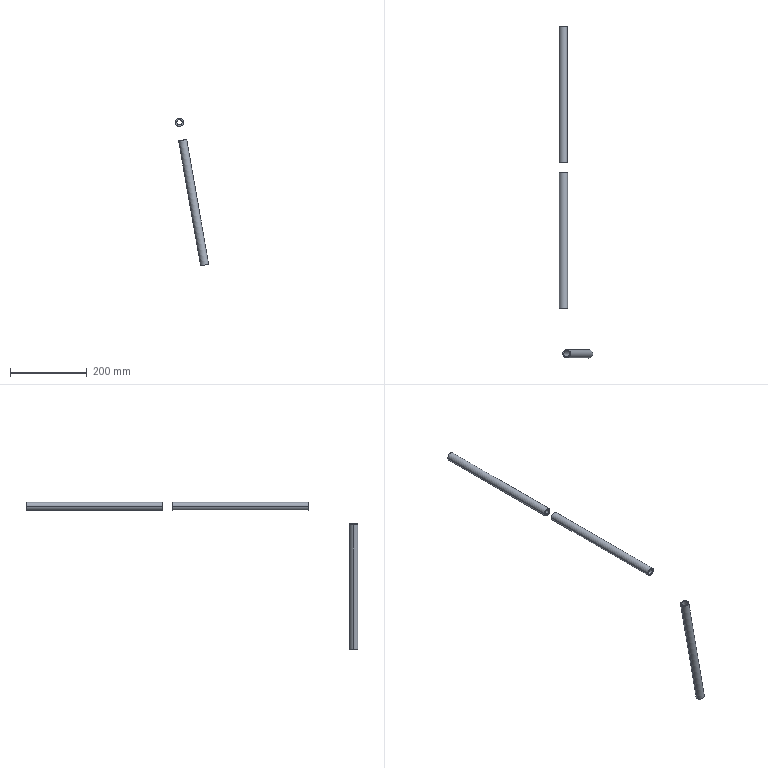Part | SolidWorks | features BaseBody 3 | 3 solids | 18 faces | box 86.694 x 862.008 x 383.174 mm | volume 199579 mm3 | cylinder 10 | plane 6 | spline 2 | commonest cylinder face diameters 21.234 x6 13.868 x2 15.234 x2
STEP:
#1=CARTESIAN_POINT('',(-12.954,392.7,7.));
#2=VERTEX_POINT('',#1);
#3=CARTESIAN_POINT('',(-12.954,392.7,-7.));
#4=VERTEX_POINT('',#3);
#5=CARTESIAN_POINT('',(-12.954,392.7,7.));
#6=CARTESIAN_POINT('',(-13.439,392.7,7.));
#7=CARTESIAN_POINT('',(-13.923,392.7,6.95));
#8=CARTESIAN_POINT('',(-14.398,392.7,6.85));
#9=CARTESIAN_POINT('',(-14.969,392.7,6.729));
#10=CARTESIAN_POINT('',(-15.523,392.7,6.538));
#11=CARTESIAN_POINT('',(-16.047,392.7,6.28));
#12=CARTESIAN_POINT('',(-16.797,392.7,5.91));
#13=CARTESIAN_POINT('',(-17.476,392.7,5.409));
#14=CARTESIAN_POINT('',(-18.049,392.7,4.8));
#15=CARTESIAN_POINT('',(-18.644,392.7,4.168));
#16=CARTESIAN_POINT('',(-19.117,392.7,3.431));
#17=CARTESIAN_POINT('',(-19.442,392.7,2.626));
#18=CARTESIAN_POINT('',(-19.78,392.7,1.792));
#19=CARTESIAN_POINT('',(-19.954,392.7,0.9002));
#20=CARTESIAN_POINT('',(-19.954,392.7,0.));
#21=CARTESIAN_POINT('',(-19.954,392.7,-0.9002));
#22=CARTESIAN_POINT('',(-19.78,392.7,-1.792));
#23=CARTESIAN_POINT('',(-19.442,392.7,-2.626));
#24=CARTESIAN_POINT('',(-19.117,392.7,-3.431));
#25=CARTESIAN_POINT('',(-18.644,392.7,-4.168));
#26=CARTESIAN_POINT('',(-18.049,392.7,-4.8));
#27=CARTESIAN_POINT('',(-17.476,392.7,-5.409));
#28=CARTESIAN_POINT('',(-16.797,392.7,-5.91));
#29=CARTESIAN_POINT('',(-16.047,392.7,-6.28));
#30=CARTESIAN_POINT('',(-15.523,392.7,-6.538));
#31=CARTESIAN_POINT('',(-14.969,392.7,-6.729));
#32=CARTESIAN_POINT('',(-14.398,392.7,-6.85));
#33=CARTESIAN_POINT('',(-13.923,392.7,-6.95));
#34=CARTESIAN_POINT('',(-13.439,392.7,-7.));
#35=CARTESIAN_POINT('',(-12.954,392.7,-7.));
#36=B_SPLINE_CURVE_WITH_KNOTS('',3,(#5,#6,#7,#8,#9,#10,#11,#12,#13,#14,#15,#16,#17,#18,#19,#20,#21,#22,#23,#24,#25,#26,#27,#28,#29,#30,#31,#32,#33,#34,#35),.UNSPECIFIED.,.F.,.F.,(4,3,3,3,3,3,3,3,3,3,4),(0.,0.1457,0.3209,0.572,0.8325,1.103,1.373,1.633,1.885,2.06,2.205),.UNSPECIFIED.);
#37=EDGE_CURVE('',#2,#4,#36,.T.);
#38=ORIENTED_EDGE('',*,*,#37,.F.);
#39=CARTESIAN_POINT('',(-12.954,392.7,-7.));
#40=CARTESIAN_POINT('',(-12.468,392.7,-7.));
#41=CARTESIAN_POINT('',(-11.984,392.7,-6.95));
#42=CARTESIAN_POINT('',(-11.509,392.7,-6.85));
#43=CARTESIAN_POINT('',(-10.938,392.7,-6.729));
#44=CARTESIAN_POINT('',(-10.384,392.7,-6.538));
#45=CARTESIAN_POINT('',(-9.86,392.7,-6.28));
#46=CARTESIAN_POINT('',(-9.11,392.7,-5.91));
#47=CARTESIAN_POINT('',(-8.432,392.7,-5.409));
#48=CARTESIAN_POINT('',(-7.858,392.7,-4.8));
#49=CARTESIAN_POINT('',(-7.263,392.7,-4.168));
#50=CARTESIAN_POINT('',(-6.79,392.7,-3.431));
#51=CARTESIAN_POINT('',(-6.465,392.7,-2.626));
#52=CARTESIAN_POINT('',(-6.127,392.7,-1.792));
#53=CARTESIAN_POINT('',(-5.953,392.7,-0.9002));
#54=CARTESIAN_POINT('',(-5.953,392.7,0.));
#55=CARTESIAN_POINT('',(-5.953,392.7,0.9002));
#56=CARTESIAN_POINT('',(-6.127,392.7,1.792));
#57=CARTESIAN_POINT('',(-6.465,392.7,2.626));
#58=CARTESIAN_POINT('',(-6.79,392.7,3.431));
#59=CARTESIAN_POINT('',(-7.263,392.7,4.168));
#60=CARTESIAN_POINT('',(-7.858,392.7,4.8));
#61=CARTESIAN_POINT('',(-8.432,392.7,5.409));
#62=CARTESIAN_POINT('',(-9.11,392.7,5.91));
#63=CARTESIAN_POINT('',(-9.86,392.7,6.28));
#64=CARTESIAN_POINT('',(-10.384,392.7,6.538));
#65=CARTESIAN_POINT('',(-10.938,392.7,6.729));
#66=CARTESIAN_POINT('',(-11.509,392.7,6.85));
#67=CARTESIAN_POINT('',(-11.984,392.7,6.95));
#68=CARTESIAN_POINT('',(-12.468,392.7,7.));
#69=CARTESIAN_POINT('',(-12.954,392.7,7.));
#70=B_SPLINE_CURVE_WITH_KNOTS('',3,(#39,#40,#41,#42,#43,#44,#45,#46,#47,#48,#49,#50,#51,#52,#53,#54,#55,#56,#57,#58,#59,#60,#61,#62,#63,#64,#65,#66,#67,#68,#69),.UNSPECIFIED.,.F.,.F.,(4,3,3,3,3,3,3,3,3,3,4),(0.,0.1457,0.3209,0.572,0.8325,1.103,1.373,1.633,1.885,2.06,2.205),.UNSPECIFIED.);
#71=EDGE_CURVE('',#4,#2,#70,.T.);
#72=ORIENTED_EDGE('',*,*,#71,.F.);
#73=EDGE_LOOP('',(#38,#72));
#74=FACE_BOUND('',#73,.T.);
#75=CARTESIAN_POINT('',(-2.337,392.7,0.));
#76=VERTEX_POINT('',#75);
#77=CARTESIAN_POINT('',(-23.571,392.7,0.));
#78=VERTEX_POINT('',#77);
#79=CARTESIAN_POINT('',(-12.954,392.7,0.));
#80=DIRECTION('',(0.,1.,0.));
#81=DIRECTION('',(1.,0.,0.));
#82=AXIS2_PLACEMENT_3D('',#79,#80,#81);
#83=CIRCLE('',#82,10.617);
#84=EDGE_CURVE('',#76,#78,#83,.T.);
#85=ORIENTED_EDGE('',*,*,#84,.F.);
#86=CARTESIAN_POINT('',(-12.954,392.7,0.));
#87=DIRECTION('',(0.,1.,0.));
#88=DIRECTION('',(-1.,0.,0.));
#89=AXIS2_PLACEMENT_3D('',#86,#87,#88);
#90=CIRCLE('',#89,10.617);
#91=EDGE_CURVE('',#78,#76,#90,.T.);
#92=ORIENTED_EDGE('',*,*,#91,.F.);
#93=EDGE_LOOP('',(#85,#92));
#94=FACE_OUTER_BOUND('',#93,.T.);
#95=CARTESIAN_POINT('',(-12.954,392.7,0.));
#96=DIRECTION('',(0.,-1.,0.));
#97=DIRECTION('',(0.,0.,-1.));
#98=AXIS2_PLACEMENT_3D('',#95,#96,#97);
#99=PLANE('',#98);
#100=ADVANCED_FACE('',(#74,#94),#99,.T.);
#101=CARTESIAN_POINT('',(-12.954,747.046,7.));
#102=VERTEX_POINT('',#101);
#103=CARTESIAN_POINT('',(-12.954,747.046,-7.));
#104=VERTEX_POINT('',#103);
#105=CARTESIAN_POINT('',(-12.954,747.046,7.));
#106=CARTESIAN_POINT('',(-12.468,747.046,7.));
#107=CARTESIAN_POINT('',(-11.984,747.046,6.95));
#108=CARTESIAN_POINT('',(-10.938,747.046,6.729));
#109=CARTESIAN_POINT('',(-10.384,747.046,6.538));
#110=CARTESIAN_POINT('',(-9.11,747.046,5.91));
#111=CARTESIAN_POINT('',(-8.432,747.046,5.409));
#112=CARTESIAN_POINT('',(-7.263,747.046,4.168));
#113=CARTESIAN_POINT('',(-6.79,747.046,3.431));
#114=CARTESIAN_POINT('',(-6.127,747.046,1.792));
#115=CARTESIAN_POINT('',(-5.953,747.046,0.9002));
#116=CARTESIAN_POINT('',(-5.953,747.046,-0.9002));
#117=CARTESIAN_POINT('',(-6.127,747.046,-1.792));
#118=CARTESIAN_POINT('',(-6.79,747.046,-3.431));
#119=CARTESIAN_POINT('',(-7.263,747.046,-4.168));
#120=CARTESIAN_POINT('',(-8.432,747.046,-5.409));
#121=CARTESIAN_POINT('',(-9.11,747.046,-5.91));
#122=CARTESIAN_POINT('',(-10.384,747.046,-6.538));
#123=CARTESIAN_POINT('',(-10.938,747.046,-6.729));
#124=CARTESIAN_POINT('',(-11.984,747.046,-6.95));
#125=CARTESIAN_POINT('',(-12.468,747.046,-7.));
#126=CARTESIAN_POINT('',(-12.954,747.046,-7.));
#127=B_SPLINE_CURVE_WITH_KNOTS('',3,(#105,#106,#107,#108,#109,#110,#111,#112,#113,#114,#115,#116,#117,#118,#119,#120,#121,#122,#123,#124,#125,#126),.UNSPECIFIED.,.F.,.F.,(4,2,2,2,2,2,2,2,2,2,4),(0.,0.1456,0.3207,0.5718,0.8321,1.102,1.372,1.633,1.884,2.059,2.204),.UNSPECIFIED.);
#128=EDGE_CURVE('',#102,#104,#127,.T.);
#129=ORIENTED_EDGE('',*,*,#128,.F.);
#130=CARTESIAN_POINT('',(-12.954,747.046,-7.));
#131=CARTESIAN_POINT('',(-13.439,747.046,-7.));
#132=CARTESIAN_POINT('',(-13.923,747.046,-6.95));
#133=CARTESIAN_POINT('',(-14.398,747.046,-6.85));
#134=CARTESIAN_POINT('',(-14.969,747.046,-6.729));
#135=CARTESIAN_POINT('',(-15.523,747.046,-6.538));
#136=CARTESIAN_POINT('',(-16.047,747.046,-6.28));
#137=CARTESIAN_POINT('',(-16.797,747.046,-5.91));
#138=CARTESIAN_POINT('',(-17.476,747.046,-5.409));
#139=CARTESIAN_POINT('',(-18.049,747.046,-4.8));
#140=CARTESIAN_POINT('',(-18.644,747.046,-4.168));
#141=CARTESIAN_POINT('',(-19.117,747.046,-3.431));
#142=CARTESIAN_POINT('',(-19.442,747.046,-2.626));
#143=CARTESIAN_POINT('',(-19.78,747.046,-1.792));
#144=CARTESIAN_POINT('',(-19.954,747.046,-0.9002));
#145=CARTESIAN_POINT('',(-19.954,747.046,0.));
#146=CARTESIAN_POINT('',(-19.954,747.046,0.9002));
#147=CARTESIAN_POINT('',(-19.78,747.046,1.792));
#148=CARTESIAN_POINT('',(-19.442,747.046,2.626));
#149=CARTESIAN_POINT('',(-19.117,747.046,3.431));
#150=CARTESIAN_POINT('',(-18.644,747.046,4.168));
#151=CARTESIAN_POINT('',(-18.049,747.046,4.8));
#152=CARTESIAN_POINT('',(-17.476,747.046,5.409));
#153=CARTESIAN_POINT('',(-16.797,747.046,5.91));
#154=CARTESIAN_POINT('',(-16.047,747.046,6.28));
#155=CARTESIAN_POINT('',(-15.523,747.046,6.538));
#156=CARTESIAN_POINT('',(-14.969,747.046,6.729));
#157=CARTESIAN_POINT('',(-14.398,747.046,6.85));
#158=CARTESIAN_POINT('',(-13.923,747.046,6.95));
#159=CARTESIAN_POINT('',(-13.439,747.046,7.));
#160=CARTESIAN_POINT('',(-12.954,747.046,7.));
#161=B_SPLINE_CURVE_WITH_KNOTS('',3,(#130,#131,#132,#133,#134,#135,#136,#137,#138,#139,#140,#141,#142,#143,#144,#145,#146,#147,#148,#149,#150,#151,#152,#153,#154,#155,#156,#157,#158,#159,#160),.UNSPECIFIED.,.F.,.F.,(4,3,3,3,3,3,3,3,3,3,4),(0.,0.1456,0.3207,0.5718,0.8321,1.102,1.372,1.633,1.884,2.059,2.204),.UNSPECIFIED.);
#162=EDGE_CURVE('',#104,#102,#161,.T.);
#163=ORIENTED_EDGE('',*,*,#162,.F.);
#164=EDGE_LOOP('',(#129,#163));
#165=FACE_BOUND('',#164,.T.);
#166=CARTESIAN_POINT('',(-2.337,747.046,0.));
#167=VERTEX_POINT('',#166);
#168=CARTESIAN_POINT('',(-23.571,747.046,0.));
#169=VERTEX_POINT('',#168);
#170=CARTESIAN_POINT('',(-12.954,747.046,0.));
#171=DIRECTION('',(0.,-1.,0.));
#172=DIRECTION('',(1.,0.,0.));
#173=AXIS2_PLACEMENT_3D('',#170,#171,#172);
#174=CIRCLE('',#173,10.617);
#175=EDGE_CURVE('',#167,#169,#174,.T.);
#176=ORIENTED_EDGE('',*,*,#175,.F.);
#177=CARTESIAN_POINT('',(-12.954,747.046,0.));
#178=DIRECTION('',(0.,-1.,0.));
#179=DIRECTION('',(-1.,0.,0.));
#180=AXIS2_PLACEMENT_3D('',#177,#178,#179);
#181=CIRCLE('',#180,10.617);
#182=EDGE_CURVE('',#169,#167,#181,.T.);
#183=ORIENTED_EDGE('',*,*,#182,.F.);
#184=EDGE_LOOP('',(#176,#183));
#185=FACE_OUTER_BOUND('',#184,.T.);
#186=CARTESIAN_POINT('',(-12.954,747.046,0.));
#187=DIRECTION('',(0.,1.,0.));
#188=DIRECTION('',(1.,0.,0.));
#189=AXIS2_PLACEMENT_3D('',#186,#187,#188);
#190=PLANE('',#189);
#191=ADVANCED_FACE('',(#165,#185),#190,.T.);
#192=ORIENTED_EDGE('',*,*,#71,.T.);
#193=CARTESIAN_POINT('',(-12.954,747.046,7.));
#194=DIRECTION('',(0.,-1.,0.));
#195=VECTOR('',#194,1000.);
#196=LINE('',#193,#195);
#197=EDGE_CURVE('',#102,#2,#196,.T.);
#198=ORIENTED_EDGE('',*,*,#197,.F.);
#199=ORIENTED_EDGE('',*,*,#128,.T.);
#200=CARTESIAN_POINT('',(-12.954,392.7,-7.));
#201=DIRECTION('',(0.,1.,0.));
#202=VECTOR('',#201,1000.);
#203=LINE('',#200,#202);
#204=EDGE_CURVE('',#4,#104,#203,.T.);
#205=ORIENTED_EDGE('',*,*,#204,.F.);
#206=EDGE_LOOP('',(#192,#198,#199,#205));
#207=FACE_OUTER_BOUND('',#206,.T.);
#208=CARTESIAN_POINT('',(-12.954,747.046,7.));
#209=CARTESIAN_POINT('',(-12.954,357.265,7.));
#210=CARTESIAN_POINT('',(-12.468,747.046,7.));
#211=CARTESIAN_POINT('',(-12.468,357.265,7.));
#212=CARTESIAN_POINT('',(-11.984,747.046,6.95));
#213=CARTESIAN_POINT('',(-11.984,357.265,6.95));
#214=CARTESIAN_POINT('',(-10.938,747.046,6.729));
#215=CARTESIAN_POINT('',(-10.938,357.265,6.729));
#216=CARTESIAN_POINT('',(-10.384,747.046,6.538));
#217=CARTESIAN_POINT('',(-10.384,357.265,6.538));
#218=CARTESIAN_POINT('',(-9.11,747.046,5.91));
#219=CARTESIAN_POINT('',(-9.11,357.265,5.91));
#220=CARTESIAN_POINT('',(-8.432,747.046,5.409));
#221=CARTESIAN_POINT('',(-8.432,357.265,5.409));
#222=CARTESIAN_POINT('',(-7.263,747.046,4.168));
#223=CARTESIAN_POINT('',(-7.263,357.265,4.168));
#224=CARTESIAN_POINT('',(-6.79,747.046,3.431));
#225=CARTESIAN_POINT('',(-6.79,357.265,3.431));
#226=CARTESIAN_POINT('',(-6.127,747.046,1.792));
#227=CARTESIAN_POINT('',(-6.127,357.265,1.792));
#228=CARTESIAN_POINT('',(-5.953,747.046,0.9002));
#229=CARTESIAN_POINT('',(-5.953,357.265,0.9002));
#230=CARTESIAN_POINT('',(-5.953,747.046,-0.9002));
#231=CARTESIAN_POINT('',(-5.953,357.265,-0.9002));
#232=CARTESIAN_POINT('',(-6.127,747.046,-1.792));
#233=CARTESIAN_POINT('',(-6.127,357.265,-1.792));
#234=CARTESIAN_POINT('',(-6.79,747.046,-3.431));
#235=CARTESIAN_POINT('',(-6.79,357.265,-3.431));
#236=CARTESIAN_POINT('',(-7.263,747.046,-4.168));
#237=CARTESIAN_POINT('',(-7.263,357.265,-4.168));
#238=CARTESIAN_POINT('',(-8.432,747.046,-5.409));
#239=CARTESIAN_POINT('',(-8.432,357.265,-5.409));
#240=CARTESIAN_POINT('',(-9.11,747.046,-5.91));
#241=CARTESIAN_POINT('',(-9.11,357.265,-5.91));
#242=CARTESIAN_POINT('',(-10.384,747.046,-6.538));
#243=CARTESIAN_POINT('',(-10.384,357.265,-6.538));
#244=CARTESIAN_POINT('',(-10.938,747.046,-6.729));
#245=CARTESIAN_POINT('',(-10.938,357.265,-6.729));
#246=CARTESIAN_POINT('',(-11.984,747.046,-6.95));
#247=CARTESIAN_POINT('',(-11.984,357.265,-6.95));
#248=CARTESIAN_POINT('',(-12.468,747.046,-7.));
#249=CARTESIAN_POINT('',(-12.468,357.265,-7.));
#250=CARTESIAN_POINT('',(-12.954,747.046,-7.));
#251=CARTESIAN_POINT('',(-12.954,357.265,-7.));
#252=B_SPLINE_SURFACE_WITH_KNOTS('',3,1,((#208,#209),(#210,#211),(#212,#213),(#214,#215),(#216,#217),(#218,#219),(#220,#221),(#222,#223),(#224,#225),(#226,#227),(#228,#229),(#230,#231),(#232,#233),(#234,#235),(#236,#237),(#238,#239),(#240,#241),(#242,#243),(#244,#245),(#246,#247),(#248,#249),(#250,#251)),.UNSPECIFIED.,.F.,.F.,.F.,(4,2,2,2,2,2,2,2,2,2,4),(2,2),(0.000001,0.1456,0.3207,0.5718,0.8321,1.102,1.372,1.633,1.884,2.059,2.204),(0.,38.978),.UNSPECIFIED.);
#253=ADVANCED_FACE('',(#207),#252,.T.);
#254=ORIENTED_EDGE('',*,*,#91,.T.);
#255=CARTESIAN_POINT('',(-2.337,747.046,0.));
#256=DIRECTION('',(0.,-1.,0.));
#257=VECTOR('',#256,1000.);
#258=LINE('',#255,#257);
#259=EDGE_CURVE('',#167,#76,#258,.T.);
#260=ORIENTED_EDGE('',*,*,#259,.F.);
#261=ORIENTED_EDGE('',*,*,#175,.T.);
#262=CARTESIAN_POINT('',(-23.571,392.7,0.));
#263=DIRECTION('',(0.,1.,0.));
#264=VECTOR('',#263,1000.);
#265=LINE('',#262,#264);
#266=EDGE_CURVE('',#78,#169,#265,.T.);
#267=ORIENTED_EDGE('',*,*,#266,.F.);
#268=EDGE_LOOP('',(#254,#260,#261,#267));
#269=FACE_OUTER_BOUND('',#268,.T.);
#270=CARTESIAN_POINT('',(-12.954,747.046,0.));
#271=DIRECTION('',(0.,-1.,0.));
#272=DIRECTION('',(1.,0.,0.));
#273=AXIS2_PLACEMENT_3D('',#270,#271,#272);
#274=CYLINDRICAL_SURFACE('',#273,10.617);
#275=ADVANCED_FACE('',(#269),#274,.T.);
#276=ORIENTED_EDGE('',*,*,#266,.T.);
#277=ORIENTED_EDGE('',*,*,#182,.T.);
#278=ORIENTED_EDGE('',*,*,#259,.T.);
#279=ORIENTED_EDGE('',*,*,#84,.T.);
#280=EDGE_LOOP('',(#276,#277,#278,#279));
#281=FACE_OUTER_BOUND('',#280,.T.);
#282=CARTESIAN_POINT('',(-12.954,747.046,0.));
#283=DIRECTION('',(0.,-1.,0.));
#284=DIRECTION('',(1.,0.,0.));
#285=AXIS2_PLACEMENT_3D('',#282,#283,#284);
#286=CYLINDRICAL_SURFACE('',#285,10.617);
#287=ADVANCED_FACE('',(#281),#286,.T.);
#288=ORIENTED_EDGE('',*,*,#37,.T.);
#289=ORIENTED_EDGE('',*,*,#204,.T.);
#290=ORIENTED_EDGE('',*,*,#162,.T.);
#291=ORIENTED_EDGE('',*,*,#197,.T.);
#292=EDGE_LOOP('',(#288,#289,#290,#291));
#293=FACE_OUTER_BOUND('',#292,.T.);
#294=CARTESIAN_POINT('',(-12.954,747.046,-7.));
#295=CARTESIAN_POINT('',(-12.954,357.265,-7.));
#296=CARTESIAN_POINT('',(-13.439,747.046,-7.));
#297=CARTESIAN_POINT('',(-13.439,357.265,-7.));
#298=CARTESIAN_POINT('',(-13.923,747.046,-6.95));
#299=CARTESIAN_POINT('',(-13.923,357.265,-6.95));
#300=CARTESIAN_POINT('',(-14.969,747.046,-6.729));
#301=CARTESIAN_POINT('',(-14.969,357.265,-6.729));
#302=CARTESIAN_POINT('',(-15.523,747.046,-6.538));
#303=CARTESIAN_POINT('',(-15.523,357.265,-6.538));
#304=CARTESIAN_POINT('',(-16.797,747.046,-5.91));
#305=CARTESIAN_POINT('',(-16.797,357.265,-5.91));
#306=CARTESIAN_POINT('',(-17.476,747.046,-5.409));
#307=CARTESIAN_POINT('',(-17.476,357.265,-5.409));
#308=CARTESIAN_POINT('',(-18.644,747.046,-4.168));
#309=CARTESIAN_POINT('',(-18.644,357.265,-4.168));
#310=CARTESIAN_POINT('',(-19.117,747.046,-3.431));
#311=CARTESIAN_POINT('',(-19.117,357.265,-3.431));
#312=CARTESIAN_POINT('',(-19.78,747.046,-1.792));
#313=CARTESIAN_POINT('',(-19.78,357.265,-1.792));
#314=CARTESIAN_POINT('',(-19.954,747.046,-0.9002));
#315=CARTESIAN_POINT('',(-19.954,357.265,-0.9002));
#316=CARTESIAN_POINT('',(-19.954,747.046,0.9002));
#317=CARTESIAN_POINT('',(-19.954,357.265,0.9002));
#318=CARTESIAN_POINT('',(-19.78,747.046,1.792));
#319=CARTESIAN_POINT('',(-19.78,357.265,1.792));
#320=CARTESIAN_POINT('',(-19.117,747.046,3.431));
#321=CARTESIAN_POINT('',(-19.117,357.265,3.431));
#322=CARTESIAN_POINT('',(-18.644,747.046,4.168));
#323=CARTESIAN_POINT('',(-18.644,357.265,4.168));
#324=CARTESIAN_POINT('',(-17.476,747.046,5.409));
#325=CARTESIAN_POINT('',(-17.476,357.265,5.409));
#326=CARTESIAN_POINT('',(-16.797,747.046,5.91));
#327=CARTESIAN_POINT('',(-16.797,357.265,5.91));
#328=CARTESIAN_POINT('',(-15.523,747.046,6.538));
#329=CARTESIAN_POINT('',(-15.523,357.265,6.538));
#330=CARTESIAN_POINT('',(-14.969,747.046,6.729));
#331=CARTESIAN_POINT('',(-14.969,357.265,6.729));
#332=CARTESIAN_POINT('',(-13.923,747.046,6.95));
#333=CARTESIAN_POINT('',(-13.923,357.265,6.95));
#334=CARTESIAN_POINT('',(-13.439,747.046,7.));
#335=CARTESIAN_POINT('',(-13.439,357.265,7.));
#336=CARTESIAN_POINT('',(-12.954,747.046,7.));
#337=CARTESIAN_POINT('',(-12.954,357.265,7.));
#338=B_SPLINE_SURFACE_WITH_KNOTS('',3,1,((#294,#295),(#296,#297),(#298,#299),(#300,#301),(#302,#303),(#304,#305),(#306,#307),(#308,#309),(#310,#311),(#312,#313),(#314,#315),(#316,#317),(#318,#319),(#320,#321),(#322,#323),(#324,#325),(#326,#327),(#328,#329),(#330,#331),(#332,#333),(#334,#335),(#336,#337)),.UNSPECIFIED.,.F.,.F.,.F.,(4,2,2,2,2,2,2,2,2,2,4),(2,2),(0.000001,0.1456,0.3207,0.5718,0.8321,1.102,1.372,1.633,1.884,2.059,2.204),(0.,38.978),.UNSPECIFIED.);
#339=ADVANCED_FACE('',(#293),#338,.T.);
#340=CLOSED_SHELL('',(#100,#191,#253,#275,#287,#339));
#341=MANIFOLD_SOLID_BREP('',#340);
#342=CARTESIAN_POINT('',(-5.766,12.7,0.));
#343=VERTEX_POINT('',#342);
#344=CARTESIAN_POINT('',(-19.634,12.7,0.));
#345=VERTEX_POINT('',#344);
#346=CARTESIAN_POINT('',(-12.7,12.7,0.));
#347=DIRECTION('',(0.,-1.,0.));
#348=DIRECTION('',(1.,0.,0.));
#349=AXIS2_PLACEMENT_3D('',#346,#347,#348);
#350=CIRCLE('',#349,6.934);
#351=EDGE_CURVE('',#343,#345,#350,.T.);
#352=ORIENTED_EDGE('',*,*,#351,.F.);
#353=CARTESIAN_POINT('',(-12.7,12.7,0.));
#354=DIRECTION('',(0.,-1.,0.));
#355=DIRECTION('',(-1.,0.,0.));
#356=AXIS2_PLACEMENT_3D('',#353,#354,#355);
#357=CIRCLE('',#356,6.934);
#358=EDGE_CURVE('',#345,#343,#357,.T.);
#359=ORIENTED_EDGE('',*,*,#358,.F.);
#360=EDGE_LOOP('',(#352,#359));
#361=FACE_BOUND('',#360,.T.);
#362=CARTESIAN_POINT('',(-2.083,12.7,0.));
#363=VERTEX_POINT('',#362);
#364=CARTESIAN_POINT('',(-23.317,12.7,0.));
#365=VERTEX_POINT('',#364);
#366=CARTESIAN_POINT('',(-12.7,12.7,0.));
#367=DIRECTION('',(0.,1.,0.));
#368=DIRECTION('',(1.,0.,0.));
#369=AXIS2_PLACEMENT_3D('',#366,#367,#368);
#370=CIRCLE('',#369,10.617);
#371=EDGE_CURVE('',#363,#365,#370,.T.);
#372=ORIENTED_EDGE('',*,*,#371,.F.);
#373=CARTESIAN_POINT('',(-12.7,12.7,0.));
#374=DIRECTION('',(0.,1.,0.));
#375=DIRECTION('',(-1.,0.,0.));
#376=AXIS2_PLACEMENT_3D('',#373,#374,#375);
#377=CIRCLE('',#376,10.617);
#378=EDGE_CURVE('',#365,#363,#377,.T.);
#379=ORIENTED_EDGE('',*,*,#378,.F.);
#380=EDGE_LOOP('',(#372,#379));
#381=FACE_OUTER_BOUND('',#380,.T.);
#382=CARTESIAN_POINT('',(-12.7,12.7,0.));
#383=DIRECTION('',(0.,-1.,0.));
#384=DIRECTION('',(0.,0.,-1.));
#385=AXIS2_PLACEMENT_3D('',#382,#383,#384);
#386=PLANE('',#385);
#387=ADVANCED_FACE('',(#361,#381),#386,.T.);
#388=CARTESIAN_POINT('',(-5.766,367.3,0.));
#389=VERTEX_POINT('',#388);
#390=CARTESIAN_POINT('',(-19.634,367.3,0.));
#391=VERTEX_POINT('',#390);
#392=CARTESIAN_POINT('',(-12.7,367.3,0.));
#393=DIRECTION('',(0.,1.,0.));
#394=DIRECTION('',(1.,0.,0.));
#395=AXIS2_PLACEMENT_3D('',#392,#393,#394);
#396=CIRCLE('',#395,6.934);
#397=EDGE_CURVE('',#389,#391,#396,.T.);
#398=ORIENTED_EDGE('',*,*,#397,.F.);
#399=CARTESIAN_POINT('',(-12.7,367.3,0.));
#400=DIRECTION('',(0.,1.,0.));
#401=DIRECTION('',(-1.,0.,0.));
#402=AXIS2_PLACEMENT_3D('',#399,#400,#401);
#403=CIRCLE('',#402,6.934);
#404=EDGE_CURVE('',#391,#389,#403,.T.);
#405=ORIENTED_EDGE('',*,*,#404,.F.);
#406=EDGE_LOOP('',(#398,#405));
#407=FACE_BOUND('',#406,.T.);
#408=CARTESIAN_POINT('',(-2.083,367.3,0.));
#409=VERTEX_POINT('',#408);
#410=CARTESIAN_POINT('',(-23.317,367.3,0.));
#411=VERTEX_POINT('',#410);
#412=CARTESIAN_POINT('',(-12.7,367.3,0.));
#413=DIRECTION('',(0.,-1.,0.));
#414=DIRECTION('',(1.,0.,0.));
#415=AXIS2_PLACEMENT_3D('',#412,#413,#414);
#416=CIRCLE('',#415,10.617);
#417=EDGE_CURVE('',#409,#411,#416,.T.);
#418=ORIENTED_EDGE('',*,*,#417,.F.);
#419=CARTESIAN_POINT('',(-12.7,367.3,0.));
#420=DIRECTION('',(0.,-1.,0.));
#421=DIRECTION('',(-1.,0.,0.));
#422=AXIS2_PLACEMENT_3D('',#419,#420,#421);
#423=CIRCLE('',#422,10.617);
#424=EDGE_CURVE('',#411,#409,#423,.T.);
#425=ORIENTED_EDGE('',*,*,#424,.F.);
#426=EDGE_LOOP('',(#418,#425));
#427=FACE_OUTER_BOUND('',#426,.T.);
#428=CARTESIAN_POINT('',(-12.7,367.3,0.));
#429=DIRECTION('',(0.,1.,0.));
#430=DIRECTION('',(1.,0.,0.));
#431=AXIS2_PLACEMENT_3D('',#428,#429,#430);
#432=PLANE('',#431);
#433=ADVANCED_FACE('',(#407,#427),#432,.T.);
#434=ORIENTED_EDGE('',*,*,#378,.T.);
#435=CARTESIAN_POINT('',(-2.083,367.3,0.));
#436=DIRECTION('',(0.,-1.,0.));
#437=VECTOR('',#436,1000.);
#438=LINE('',#435,#437);
#439=EDGE_CURVE('',#409,#363,#438,.T.);
#440=ORIENTED_EDGE('',*,*,#439,.F.);
#441=ORIENTED_EDGE('',*,*,#417,.T.);
#442=CARTESIAN_POINT('',(-23.317,12.7,0.));
#443=DIRECTION('',(0.,1.,0.));
#444=VECTOR('',#443,1000.);
#445=LINE('',#442,#444);
#446=EDGE_CURVE('',#365,#411,#445,.T.);
#447=ORIENTED_EDGE('',*,*,#446,.F.);
#448=EDGE_LOOP('',(#434,#440,#441,#447));
#449=FACE_OUTER_BOUND('',#448,.T.);
#450=CARTESIAN_POINT('',(-12.7,367.3,0.));
#451=DIRECTION('',(0.,-1.,0.));
#452=DIRECTION('',(1.,0.,0.));
#453=AXIS2_PLACEMENT_3D('',#450,#451,#452);
#454=CYLINDRICAL_SURFACE('',#453,10.617);
#455=ADVANCED_FACE('',(#449),#454,.T.);
#456=ORIENTED_EDGE('',*,*,#446,.T.);
#457=ORIENTED_EDGE('',*,*,#424,.T.);
#458=ORIENTED_EDGE('',*,*,#439,.T.);
#459=ORIENTED_EDGE('',*,*,#371,.T.);
#460=EDGE_LOOP('',(#456,#457,#458,#459));
#461=FACE_OUTER_BOUND('',#460,.T.);
#462=CARTESIAN_POINT('',(-12.7,367.3,0.));
#463=DIRECTION('',(0.,-1.,0.));
#464=DIRECTION('',(1.,0.,0.));
#465=AXIS2_PLACEMENT_3D('',#462,#463,#464);
#466=CYLINDRICAL_SURFACE('',#465,10.617);
#467=ADVANCED_FACE('',(#461),#466,.T.);
#468=ORIENTED_EDGE('',*,*,#358,.T.);
#469=CARTESIAN_POINT('',(-5.766,367.3,0.));
#470=DIRECTION('',(0.,-1.,0.));
#471=VECTOR('',#470,1000.);
#472=LINE('',#469,#471);
#473=EDGE_CURVE('',#389,#343,#472,.T.);
#474=ORIENTED_EDGE('',*,*,#473,.F.);
#475=ORIENTED_EDGE('',*,*,#397,.T.);
#476=CARTESIAN_POINT('',(-19.634,12.7,0.));
#477=DIRECTION('',(0.,1.,0.));
#478=VECTOR('',#477,1000.);
#479=LINE('',#476,#478);
#480=EDGE_CURVE('',#345,#391,#479,.T.);
#481=ORIENTED_EDGE('',*,*,#480,.F.);
#482=EDGE_LOOP('',(#468,#474,#475,#481));
#483=FACE_OUTER_BOUND('',#482,.T.);
#484=CARTESIAN_POINT('',(-12.7,367.3,0.));
#485=DIRECTION('',(0.,-1.,0.));
#486=DIRECTION('',(1.,0.,0.));
#487=AXIS2_PLACEMENT_3D('',#484,#485,#486);
#488=CYLINDRICAL_SURFACE('',#487,6.934);
#489=ADVANCED_FACE('',(#483),#488,.F.);
#490=ORIENTED_EDGE('',*,*,#480,.T.);
#491=ORIENTED_EDGE('',*,*,#404,.T.);
#492=ORIENTED_EDGE('',*,*,#473,.T.);
#493=ORIENTED_EDGE('',*,*,#351,.T.);
#494=EDGE_LOOP('',(#490,#491,#492,#493));
#495=FACE_OUTER_BOUND('',#494,.T.);
#496=CARTESIAN_POINT('',(-12.7,367.3,0.));
#497=DIRECTION('',(0.,-1.,0.));
#498=DIRECTION('',(1.,0.,0.));
#499=AXIS2_PLACEMENT_3D('',#496,#497,#498);
#500=CYLINDRICAL_SURFACE('',#499,6.934);
#501=ADVANCED_FACE('',(#495),#500,.F.);
#502=CLOSED_SHELL('',(#387,#433,#455,#467,#489,#501));
#503=MANIFOLD_SOLID_BREP('',#502);
#504=CARTESIAN_POINT('',(45.165,-104.345,-372.036));
#505=VERTEX_POINT('',#504);
#506=CARTESIAN_POINT('',(60.168,-104.345,-369.391));
#507=VERTEX_POINT('',#506);
#508=CARTESIAN_POINT('',(52.667,-104.345,-370.713));
#509=DIRECTION('',(0.1736,0.,-0.9848));
#510=DIRECTION('',(-0.9848,0.,-0.1736));
#511=AXIS2_PLACEMENT_3D('',#508,#509,#510);
#512=CIRCLE('',#511,7.617);
#513=EDGE_CURVE('',#505,#507,#512,.T.);
#514=ORIENTED_EDGE('',*,*,#513,.F.);
#515=CARTESIAN_POINT('',(52.667,-104.345,-370.713));
#516=DIRECTION('',(0.1736,0.,-0.9848));
#517=DIRECTION('',(0.9848,0.,0.1736));
#518=AXIS2_PLACEMENT_3D('',#515,#516,#517);
#519=CIRCLE('',#518,7.617);
#520=EDGE_CURVE('',#507,#505,#519,.T.);
#521=ORIENTED_EDGE('',*,*,#520,.F.);
#522=EDGE_LOOP('',(#514,#521));
#523=FACE_BOUND('',#522,.T.);
#524=CARTESIAN_POINT('',(42.211,-104.345,-372.557));
#525=VERTEX_POINT('',#524);
#526=CARTESIAN_POINT('',(63.123,-104.345,-368.87));
#527=VERTEX_POINT('',#526);
#528=CARTESIAN_POINT('',(52.667,-104.345,-370.713));
#529=DIRECTION('',(-0.1736,0.,0.9848));
#530=DIRECTION('',(-0.9848,0.,-0.1736));
#531=AXIS2_PLACEMENT_3D('',#528,#529,#530);
#532=CIRCLE('',#531,10.617);
#533=EDGE_CURVE('',#525,#527,#532,.T.);
#534=ORIENTED_EDGE('',*,*,#533,.F.);
#535=CARTESIAN_POINT('',(52.667,-104.345,-370.713));
#536=DIRECTION('',(-0.1736,0.,0.9848));
#537=DIRECTION('',(0.9848,0.,0.1736));
#538=AXIS2_PLACEMENT_3D('',#535,#536,#537);
#539=CIRCLE('',#538,10.617);
#540=EDGE_CURVE('',#527,#525,#539,.T.);
#541=ORIENTED_EDGE('',*,*,#540,.F.);
#542=EDGE_LOOP('',(#534,#541));
#543=FACE_OUTER_BOUND('',#542,.T.);
#544=CARTESIAN_POINT('',(52.667,-104.345,-370.713));
#545=DIRECTION('',(0.1736,0.,-0.9848));
#546=DIRECTION('',(0.,-1.,0.));
#547=AXIS2_PLACEMENT_3D('',#544,#545,#546);
#548=PLANE('',#547);
#549=ADVANCED_FACE('',(#523,#543),#548,.T.);
#550=CARTESIAN_POINT('',(-12.05,-104.345,-47.55));
#551=VERTEX_POINT('',#550);
#552=CARTESIAN_POINT('',(2.953,-104.345,-44.905));
#553=VERTEX_POINT('',#552);
#554=CARTESIAN_POINT('',(-4.549,-104.345,-46.228));
#555=DIRECTION('',(-0.1736,0.,0.9848));
#556=DIRECTION('',(-0.9848,0.,-0.1736));
#557=AXIS2_PLACEMENT_3D('',#554,#555,#556);
#558=CIRCLE('',#557,7.617);
#559=EDGE_CURVE('',#551,#553,#558,.T.);
#560=ORIENTED_EDGE('',*,*,#559,.F.);
#561=CARTESIAN_POINT('',(-4.549,-104.345,-46.228));
#562=DIRECTION('',(-0.1736,0.,0.9848));
#563=DIRECTION('',(0.9848,0.,0.1736));
#564=AXIS2_PLACEMENT_3D('',#561,#562,#563);
#565=CIRCLE('',#564,7.617);
#566=EDGE_CURVE('',#553,#551,#565,.T.);
#567=ORIENTED_EDGE('',*,*,#566,.F.);
#568=EDGE_LOOP('',(#560,#567));
#569=FACE_BOUND('',#568,.T.);
#570=CARTESIAN_POINT('',(-15.005,-104.345,-48.071));
#571=VERTEX_POINT('',#570);
#572=CARTESIAN_POINT('',(5.907,-104.345,-44.384));
#573=VERTEX_POINT('',#572);
#574=CARTESIAN_POINT('',(-4.549,-104.345,-46.228));
#575=DIRECTION('',(0.1736,0.,-0.9848));
#576=DIRECTION('',(-0.9848,0.,-0.1736));
#577=AXIS2_PLACEMENT_3D('',#574,#575,#576);
#578=CIRCLE('',#577,10.617);
#579=EDGE_CURVE('',#571,#573,#578,.T.);
#580=ORIENTED_EDGE('',*,*,#579,.F.);
#581=CARTESIAN_POINT('',(-4.549,-104.345,-46.228));
#582=DIRECTION('',(0.1736,0.,-0.9848));
#583=DIRECTION('',(0.9848,0.,0.1736));
#584=AXIS2_PLACEMENT_3D('',#581,#582,#583);
#585=CIRCLE('',#584,10.617);
#586=EDGE_CURVE('',#573,#571,#585,.T.);
#587=ORIENTED_EDGE('',*,*,#586,.F.);
#588=EDGE_LOOP('',(#580,#587));
#589=FACE_OUTER_BOUND('',#588,.T.);
#590=CARTESIAN_POINT('',(-4.549,-104.345,-46.228));
#591=DIRECTION('',(-0.1736,0.,0.9848));
#592=DIRECTION('',(0.,1.,0.));
#593=AXIS2_PLACEMENT_3D('',#590,#591,#592);
#594=PLANE('',#593);
#595=ADVANCED_FACE('',(#569,#589),#594,.T.);
#596=ORIENTED_EDGE('',*,*,#540,.T.);
#597=CARTESIAN_POINT('',(-15.005,-104.345,-48.071));
#598=DIRECTION('',(0.1736,0.,-0.9848));
#599=VECTOR('',#598,1000.);
#600=LINE('',#597,#599);
#601=EDGE_CURVE('',#571,#525,#600,.T.);
#602=ORIENTED_EDGE('',*,*,#601,.F.);
#603=ORIENTED_EDGE('',*,*,#579,.T.);
#604=CARTESIAN_POINT('',(63.123,-104.345,-368.87));
#605=DIRECTION('',(-0.1736,0.,0.9848));
#606=VECTOR('',#605,1000.);
#607=LINE('',#604,#606);
#608=EDGE_CURVE('',#527,#573,#607,.T.);
#609=ORIENTED_EDGE('',*,*,#608,.F.);
#610=EDGE_LOOP('',(#596,#602,#603,#609));
#611=FACE_OUTER_BOUND('',#610,.T.);
#612=CARTESIAN_POINT('',(-4.549,-104.345,-46.228));
#613=DIRECTION('',(0.1736,0.,-0.9848));
#614=DIRECTION('',(-0.9848,0.,-0.1736));
#615=AXIS2_PLACEMENT_3D('',#612,#613,#614);
#616=CYLINDRICAL_SURFACE('',#615,10.617);
#617=ADVANCED_FACE('',(#611),#616,.T.);
#618=ORIENTED_EDGE('',*,*,#608,.T.);
#619=ORIENTED_EDGE('',*,*,#586,.T.);
#620=ORIENTED_EDGE('',*,*,#601,.T.);
#621=ORIENTED_EDGE('',*,*,#533,.T.);
#622=EDGE_LOOP('',(#618,#619,#620,#621));
#623=FACE_OUTER_BOUND('',#622,.T.);
#624=CARTESIAN_POINT('',(-4.549,-104.345,-46.228));
#625=DIRECTION('',(0.1736,0.,-0.9848));
#626=DIRECTION('',(-0.9848,0.,-0.1736));
#627=AXIS2_PLACEMENT_3D('',#624,#625,#626);
#628=CYLINDRICAL_SURFACE('',#627,10.617);
#629=ADVANCED_FACE('',(#623),#628,.T.);
#630=ORIENTED_EDGE('',*,*,#520,.T.);
#631=CARTESIAN_POINT('',(-12.05,-104.345,-47.55));
#632=DIRECTION('',(0.1736,0.,-0.9848));
#633=VECTOR('',#632,1000.);
#634=LINE('',#631,#633);
#635=EDGE_CURVE('',#551,#505,#634,.T.);
#636=ORIENTED_EDGE('',*,*,#635,.F.);
#637=ORIENTED_EDGE('',*,*,#559,.T.);
#638=CARTESIAN_POINT('',(60.168,-104.345,-369.391));
#639=DIRECTION('',(-0.1736,0.,0.9848));
#640=VECTOR('',#639,1000.);
#641=LINE('',#638,#640);
#642=EDGE_CURVE('',#507,#553,#641,.T.);
#643=ORIENTED_EDGE('',*,*,#642,.F.);
#644=EDGE_LOOP('',(#630,#636,#637,#643));
#645=FACE_OUTER_BOUND('',#644,.T.);
#646=CARTESIAN_POINT('',(-4.549,-104.345,-46.228));
#647=DIRECTION('',(0.1736,0.,-0.9848));
#648=DIRECTION('',(-0.9848,0.,-0.1736));
#649=AXIS2_PLACEMENT_3D('',#646,#647,#648);
#650=CYLINDRICAL_SURFACE('',#649,7.617);
#651=ADVANCED_FACE('',(#645),#650,.F.);
#652=ORIENTED_EDGE('',*,*,#642,.T.);
#653=ORIENTED_EDGE('',*,*,#566,.T.);
#654=ORIENTED_EDGE('',*,*,#635,.T.);
#655=ORIENTED_EDGE('',*,*,#513,.T.);
#656=EDGE_LOOP('',(#652,#653,#654,#655));
#657=FACE_OUTER_BOUND('',#656,.T.);
#658=CARTESIAN_POINT('',(-4.549,-104.345,-46.228));
#659=DIRECTION('',(0.1736,0.,-0.9848));
#660=DIRECTION('',(-0.9848,0.,-0.1736));
#661=AXIS2_PLACEMENT_3D('',#658,#659,#660);
#662=CYLINDRICAL_SURFACE('',#661,7.617);
#663=ADVANCED_FACE('',(#657),#662,.F.);
#664=CLOSED_SHELL('',(#549,#595,#617,#629,#651,#663));
#665=MANIFOLD_SOLID_BREP('',#664);
#666=CARTESIAN_POINT('',(0.,0.,0.));
#667=DIRECTION('',(0.,0.,1.));
#668=DIRECTION('',(1.,0.,0.));
#669=AXIS2_PLACEMENT_3D('',#666,#667,#668);
#670=(LENGTH_UNIT()NAMED_UNIT(*)SI_UNIT(.MILLI.,.METRE.));
#671=UNCERTAINTY_MEASURE_WITH_UNIT(LENGTH_MEASURE(0.00001),#670,'','');
#672=(NAMED_UNIT(*)PLANE_ANGLE_UNIT()SI_UNIT($,.RADIAN.));
#673=(NAMED_UNIT(*)SI_UNIT($,.STERADIAN.)SOLID_ANGLE_UNIT());
#674=(GEOMETRIC_REPRESENTATION_CONTEXT(3)GLOBAL_UNCERTAINTY_ASSIGNED_CONTEXT((#671))GLOBAL_UNIT_ASSIGNED_CONTEXT((#670,#672,#673))REPRESENTATION_CONTEXT('',''));
#675=ADVANCED_BREP_SHAPE_REPRESENTATION('',(#341,#503,#665,#669),#674);